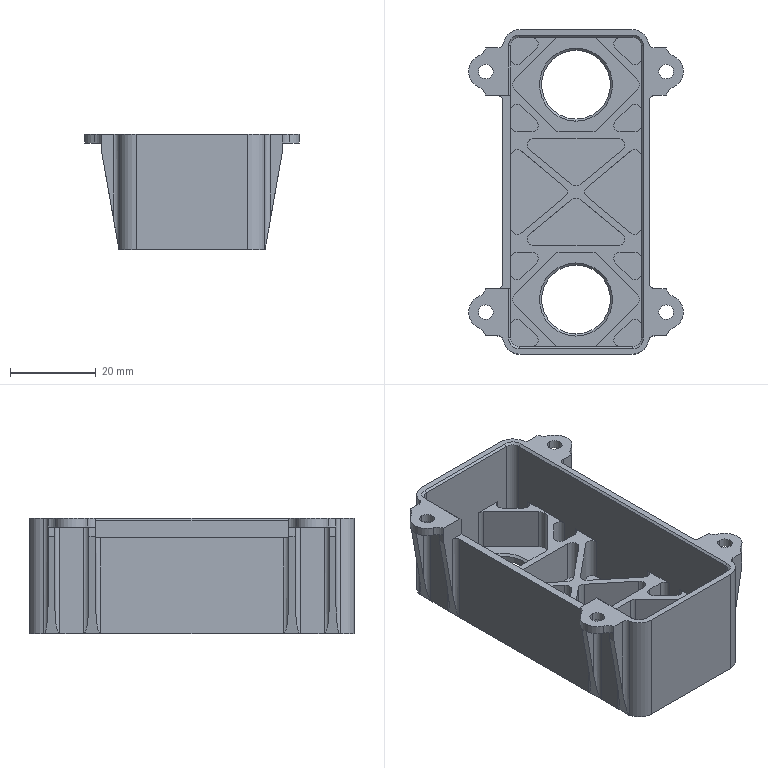NC program | NX | posted with a generic post | part box 50 x 75.58 x 26.8 mm
Lines 71 to 1246 of 35818:
(FLOOR_WALL , TOOL : D10)
N128 T15 M6
N130 G54
N132 G17 G0 G90 X23. Y1.305 S9500 M3
N134 G43 Z30. H15
N136 Z0.6
N138 G94 G1 Z-0.4 F1000.
N140 X22.357 Y0.766
N142 G3 X22. Y0. R1.
N144 G1 Y-17.499 F2000.
N146 G3 X21. Y-17.4 R5.1
N148 G1 X10.2
N150 Y17.4
N152 X21.
N154 G3 X22. Y17.499 R5.1
N156 G1 Y0.
N158 X17.
N160 Y-12.4
N162 X15.2
N164 Y12.4
N166 X17.
N168 Y0.
N170 G3 X17.357 Y-0.766 R1.
N172 G1 Z0.6
N174 G0 X23. Y1.305 Z0.2
N176 G1 Z-0.8 F1000.
N178 X22.357 Y0.766
N180 G3 X22. Y0. R1.
N182 G1 Y-17.499 F2000.
N184 G3 X21. Y-17.4 R5.1
N186 G1 X10.2
N188 Y17.4
N190 X21.
N192 G3 X22. Y17.499 R5.1
N194 G1 Y0.
N196 X17.
N198 Y-12.4
N200 X15.2
N202 Y12.4
N204 X17.
N206 Y0.
N208 G3 X17.357 Y-0.766 R1.
N210 G1 Z0.2
N212 G0 X23. Y1.305 Z-0.2
N214 G1 Z-1.2 F1000.
N216 X22.357 Y0.766
N218 G3 X22. Y0. R1.
N220 G1 Y-17.499 F2000.
N222 G3 X21. Y-17.4 R5.1
N224 G1 X10.2
N226 Y17.4
N228 X21.
N230 G3 X22. Y17.499 R5.1
N232 G1 Y0.
N234 X17.
N236 Y-12.4
N238 X15.2
N240 Y12.4
N242 X17.
N244 Y0.
N246 G3 X17.357 Y-0.766 R1.
N248 G1 Z-0.2
N250 G0 X23. Y1.305 Z-0.6
N252 G1 Z-1.6 F1000.
N254 X22.357 Y0.766
N256 G3 X22. Y0. R1.
N258 G1 Y-17.499 F2000.
N260 G3 X21. Y-17.4 R5.1
N262 G1 X10.2
N264 Y17.4
N266 X21.
N268 G3 X22. Y17.499 R5.1
N270 G1 Y0.
N272 X17.
N274 Y-12.4
N276 X15.2
N278 Y12.4
N280 X17.
N282 Y0.
N284 G3 X17.357 Y-0.766 R1.
N286 G1 Z-0.6
N288 G0 X23. Y1.305 Z-1.
N290 G1 Z-2. F1000.
N292 X22.357 Y0.766
N294 G3 X22. Y0. R1.
N296 G1 Y-17.499 F2000.
N298 G3 X21. Y-17.4 R5.1
N300 G1 X10.2
N302 Y17.4
N304 X21.
N306 G3 X22. Y17.499 R5.1
N308 G1 Y0.
N310 X17.
N312 Y-12.4
N314 X15.2
N316 Y12.4
N318 X17.
N320 Y0.
N322 G3 X17.357 Y-0.766 R1.
N324 G1 Z-1.
N326 G0 X23. Y1.305 Z-1.4
N328 G1 Z-2.4 F1000.
N330 X22.357 Y0.766
N332 G3 X22. Y0. R1.
N334 G1 Y-17.499 F2000.
N336 G3 X21. Y-17.4 R5.1
N338 G1 X10.2
N340 Y17.4
N342 X21.
N344 G3 X22. Y17.499 R5.1
N346 G1 Y0.
N348 X17.
N350 Y-12.4
N352 X15.2
N354 Y12.4
N356 X17.
N358 Y0.
N360 G3 X17.357 Y-0.766 R1.
N362 G1 Z-1.4
N364 G0 X23. Y1.305 Z-1.8
N366 G1 Z-2.8 F1000.
N368 X22.357 Y0.766
N370 G3 X22. Y0. R1.
N372 G1 Y-17.499 F2000.
N374 G3 X21. Y-17.4 R5.1
N376 G1 X10.2
N378 Y17.4
N380 X21.
N382 G3 X22. Y17.499 R5.1
N384 G1 Y0.
N386 X17.
N388 Y-12.4
N390 X15.2
N392 Y12.4
N394 X17.
N396 Y0.
N398 G3 X17.357 Y-0.766 R1.
N400 G1 Z-1.8
N402 G0 X23. Y1.305 Z-2.2
N404 G1 Z-3.2 F1000.
N406 X22.357 Y0.766
N408 G3 X22. Y0. R1.
N410 G1 Y-17.499 F2000.
N412 G3 X21. Y-17.4 R5.1
N414 G1 X10.2
N416 Y17.4
N418 X21.
N420 G3 X22. Y17.499 R5.1
N422 G1 Y0.
N424 X17.
N426 Y-12.4
N428 X15.2
N430 Y12.4
N432 X17.
N434 Y0.
N436 G3 X17.357 Y-0.766 R1.
N438 G1 Z-2.2
N440 G0 X23. Y1.305 Z-2.6
N442 G1 Z-3.6 F1000.
N444 X22.357 Y0.766
N446 G3 X22. Y0. R1.
N448 G1 Y-17.499 F2000.
N450 G3 X21. Y-17.4 R5.1
N452 G1 X10.2
N454 Y17.4
N456 X21.
N458 G3 X22. Y17.499 R5.1
N460 G1 Y0.
N462 X17.
N464 Y-12.4
N466 X15.2
N468 Y12.4
N470 X17.
N472 Y0.
N474 G3 X17.357 Y-0.766 R1.
N476 G1 Z-2.6
N478 G0 X23. Y1.305 Z-3.
N480 G1 Z-4. F1000.
N482 X22.357 Y0.766
N484 G3 X22. Y0. R1.
N486 G1 Y-17.499 F2000.
N488 G3 X21. Y-17.4 R5.1
N490 G1 X10.2
N492 Y17.4
N494 X21.
N496 G3 X22. Y17.499 R5.1
N498 G1 Y0.
N500 X17.
N502 Y-12.4
N504 X15.2
N506 Y12.4
N508 X17.
N510 Y0.
N512 G3 X17.357 Y-0.766 R1.
N514 G1 Z-3.
N516 G0 X23. Y1.305 Z-3.4
N518 G1 Z-4.4 F1000.
N520 X22.357 Y0.766
N522 G3 X22. Y0. R1.
N524 G1 Y-17.499 F2000.
N526 G3 X21. Y-17.4 R5.1
N528 G1 X10.2
N530 Y17.4
N532 X21.
N534 G3 X22. Y17.499 R5.1
N536 G1 Y0.
N538 X17.
N540 Y-12.4
N542 X15.2
N544 Y12.4
N546 X17.
N548 Y0.
N550 G3 X17.357 Y-0.766 R1.
N552 G1 Z-3.4
N554 G0 Z30.
(CAVITY_MILL_COPY_1 , TOOL : D10)
N556 X3.7 Y3.037
N558 Z1.5
N560 G1 Y9.845 Z1.143 F1000.
N562 X2.95 Y10.526 Z1.09
N564 X2.537 Y10.964 Z1.059
N566 X1.9 Y11.752 Z1.005
N568 Y-11.752 Z-0.226
N570 X2.537 Y-10.964 Z-0.279
N572 X2.95 Y-10.526 Z-0.311
N574 X3.7 Y-9.845 Z-0.364
N576 Y0. Z-0.88
N578 Y9.845 F2500.
N580 G2 X1.9 Y11.752 R17.1
N582 G1 Y-11.752
N584 G2 X3.7 Y-9.845 R17.1
N586 G1 Y0.
N588 X9.7
N590 Y12.858
N592 G2 X4.1 Y22.5 R11.1
N594 G1 Y24.89
N596 X-4.1
N598 Y-24.89
N600 X4.1
N602 Y-22.5
N604 G2 X9.7 Y-12.858 R11.1
N606 G1 Y0.
N608 X15.7
N610 Y17.4
N612 X15.2
N614 G2 X10.1 Y22.5 R5.1
N616 G1 Y30.89
N618 X-10.1
N620 Y-30.89
N622 X10.1
N624 Y-22.5
N626 G2 X15.2 Y-17.4 R5.1
N628 G1 X15.7
N630 Y0.
N632 G2 X16.2 Y0.866 R1.
N634 G1 Z0.12
N636 G0 Z30.
N638 X3.7 Y3.037
N640 Z0.62
N642 G1 Y9.845 Z0.263 F1000.
N644 X2.95 Y10.526 Z0.21
N646 X2.537 Y10.964 Z0.179
N648 X1.9 Y11.752 Z0.125
N650 Y-11.752 Z-1.106
N652 X2.537 Y-10.964 Z-1.159
N654 X2.95 Y-10.526 Z-1.191
N656 X3.7 Y-9.845 Z-1.244
N658 Y0. Z-1.76
N660 Y9.845 F2500.
N662 G2 X1.9 Y11.752 R17.1
N664 G1 Y-11.752
N666 G2 X3.7 Y-9.845 R17.1
N668 G1 Y0.
N670 X9.7
N672 Y12.858
N674 G2 X4.1 Y22.5 R11.1
N676 G1 Y24.89
N678 X-4.1
N680 Y-24.89
N682 X4.1
N684 Y-22.5
N686 G2 X9.7 Y-12.858 R11.1
N688 G1 Y0.
N690 X15.7
N692 Y17.4
N694 X15.2
N696 G2 X10.1 Y22.5 R5.1
N698 G1 Y30.89
N700 X-10.1
N702 Y-30.89
N704 X10.1
N706 Y-22.5
N708 G2 X15.2 Y-17.4 R5.1
N710 G1 X15.7
N712 Y0.
N714 G2 X16.2 Y0.866 R1.
N716 G1 Z-0.76
N718 G0 X3.7 Y3.037 Z-0.26
N720 G1 Y9.845 Z-0.617 F1000.
N722 X2.95 Y10.526 Z-0.67
N724 X2.537 Y10.964 Z-0.701
N726 X1.9 Y11.752 Z-0.755
N728 Y-11.752 Z-1.986
N730 X2.537 Y-10.964 Z-2.039
N732 X2.95 Y-10.526 Z-2.071
N734 X3.7 Y-9.845 Z-2.124
N736 Y0. Z-2.64
N738 Y9.845 F2500.
N740 G2 X1.9 Y11.752 R17.1
N742 G1 Y-11.752
N744 G2 X3.7 Y-9.845 R17.1
N746 G1 Y0.
N748 X9.7
N750 Y12.858
N752 G2 X4.1 Y22.5 R11.1
N754 G1 Y24.89
N756 X-4.1
N758 Y-24.89
N760 X4.1
N762 Y-22.5
N764 G2 X9.7 Y-12.858 R11.1
N766 G1 Y0.
N768 X15.7
N770 Y17.4
N772 X15.2
N774 G2 X10.1 Y22.5 R5.1
N776 G1 Y30.89
N778 X-10.1
N780 Y-30.89
N782 X10.1
N784 Y-22.5
N786 G2 X15.2 Y-17.4 R5.1
N788 G1 X15.7
N790 Y0.
N792 G2 X16.2 Y0.866 R1.
N794 G1 Z-1.64
N796 G0 X3.7 Y3.037 Z-1.14
N798 G1 Y9.845 Z-1.497 F1000.
N800 X2.95 Y10.526 Z-1.55
N802 X2.537 Y10.964 Z-1.581
N804 X1.9 Y11.752 Z-1.635
N806 Y-11.752 Z-2.866
N808 X2.537 Y-10.964 Z-2.919
N810 X2.95 Y-10.526 Z-2.951
N812 X3.7 Y-9.845 Z-3.004
N814 Y0. Z-3.52
N816 Y9.845 F2500.
N818 G2 X1.9 Y11.752 R17.1
N820 G1 Y-11.752
N822 G2 X3.7 Y-9.845 R17.1
N824 G1 Y0.
N826 X9.7
N828 Y12.858
N830 G2 X4.1 Y22.5 R11.1
N832 G1 Y24.89
N834 X-4.1
N836 Y-24.89
N838 X4.1
N840 Y-22.5
N842 G2 X9.7 Y-12.858 R11.1
N844 G1 Y0.
N846 X15.7
N848 Y17.4
N850 X15.2
N852 G2 X10.1 Y22.5 R5.1
N854 G1 Y30.89
N856 X-10.1
N858 Y-30.89
N860 X10.1
N862 Y-22.5
N864 G2 X15.2 Y-17.4 R5.1
N866 G1 X15.7
N868 Y0.
N870 G2 X16.2 Y0.866 R1.
N872 G1 Z-2.52
N874 G0 X3.7 Y3.037 Z-2.02
N876 G1 Y9.845 Z-2.377 F1000.
N878 X2.95 Y10.526 Z-2.43
N880 X2.537 Y10.964 Z-2.461
N882 X1.9 Y11.752 Z-2.515
N884 Y-11.752 Z-3.746
N886 X2.537 Y-10.964 Z-3.799
N888 X2.95 Y-10.526 Z-3.831
N890 X3.7 Y-9.845 Z-3.884
N892 Y0. Z-4.4
N894 Y9.845 F2500.
N896 G2 X1.9 Y11.752 R17.1
N898 G1 Y-11.752
N900 G2 X3.7 Y-9.845 R17.1
N902 G1 Y0.
N904 X9.7
N906 Y12.858
N908 G2 X4.1 Y22.5 R11.1
N910 G1 Y24.89
N912 X-4.1
N914 Y-24.89
N916 X4.1
N918 Y-22.5
N920 G2 X9.7 Y-12.858 R11.1
N922 G1 Y0.
N924 X15.7
N926 Y17.4
N928 X15.2
N930 G2 X10.1 Y22.5 R5.1
N932 G1 Y30.89
N934 X-10.1
N936 Y-30.89
N938 X10.1
N940 Y-22.5
N942 G2 X15.2 Y-17.4 R5.1
N944 G1 X15.7
N946 Y0.
N948 G2 X16.2 Y0.866 R1.
N950 G1 Z-3.4
N952 G0 X4.1 Y11.491 Z-2.9
N954 G1 Y24.89 Z-3.602 F1000.
N956 X-4.1 Z-4.032
N958 Y0. Z-5.336
N960 Y-24.89 F2500.
N962 X4.1
N964 Y24.89
N966 X-4.1
N968 Y0.
N970 X-10.1
N972 Y-30.89
N974 X10.1
N976 Y30.89
N978 X-10.1
N980 Y0.
N982 G3 X-9.6 Y-0.866 R1.
N984 G1 Z-4.336
N986 G0 X4.1 Y11.491 Z-3.836
N988 G1 Y24.89 Z-4.539 F1000.
N990 X-4.1 Z-4.968
N992 Y0. Z-6.273
N994 Y-24.89 F2500.
N996 X4.1
N998 Y24.89
N1000 X-4.1
N1002 Y0.
N1004 X-10.1
N1006 Y-30.89
N1008 X10.1
N1010 Y30.89
N1012 X-10.1
N1014 Y0.
N1016 G3 X-9.6 Y-0.866 R1.
N1018 G1 Z-5.273
N1020 G0 X4.1 Y11.497 Z-4.773
N1022 G1 Y24.89 Z-5.475 F1000.
N1024 X-4.1 Z-5.904
N1026 Y7.945 Z-6.792
N1028 X-4.04 Y7.337 Z-6.824
N1030 X-4.1 Y6.739 Z-6.856
N1032 Y0. Z-7.209
N1034 Y-6.739 F2500.
N1036 G2 X-4.1 Y-7.945 R6.
N1038 G1 Y-24.89
N1040 X4.1
N1042 Y24.89
N1044 X-4.1
N1046 Y7.945
N1048 G2 X-4.1 Y6.739 R6.
N1050 G1 Y0.
N1052 X-10.1
N1054 Y-7.242
N1056 X-10.07 Y-7.342
N1058 X-10.1 Y-7.39
N1060 Y-30.89
N1062 X10.1
N1064 Y30.89
N1066 X-10.1
N1068 Y7.39
N1070 X-10.07 Y7.342
N1072 X-10.1 Y7.242
N1074 Y0.
N1076 G3 X-9.6 Y-0.866 R1.
N1078 G1 Z-6.209
N1080 G0 X4.1 Y11.498 Z-5.709
N1082 G1 Y24.89 Z-6.411 F1000.
N1084 X-4.1 Z-6.841
N1086 Y7.987 Z-7.727
N1088 X-4.035 Y7.389 Z-7.758
N1090 Y7.295 Z-7.763
N1092 X-4.1 Y6.698 Z-7.794
N1094 Y0. Z-8.145
N1096 Y-6.698 F2500.
N1098 G2 X-4.1 Y-7.987 R6.
N1100 G1 Y-24.89
N1102 X4.1
N1104 Y24.89
N1106 X-4.1
N1108 Y7.987
N1110 G2 X-4.1 Y6.698 R6.
N1112 G1 Y0.
N1114 X-10.1
N1116 Y-7.242
N1118 X-10.065 Y-7.342
N1120 X-10.1 Y-7.39
N1122 Y-30.89
N1124 X10.1
N1126 Y30.89
N1128 X-10.1
N1130 Y7.39
N1132 X-10.065 Y7.342
N1134 X-10.1 Y7.242
N1136 Y0.
N1138 G3 X-9.6 Y-0.866 R1.
N1140 G1 Z-7.145
N1142 G0 X-4.1 Y-11.491 Z-6.645
N1144 G1 Y-24.89 Z-7.348 F1000.
N1146 X4.1 Z-7.777
N1148 Y0. Z-9.082
N1150 Y24.89 F2500.
N1152 X-4.1
N1154 Y8.025
N1156 G2 X-4.1 Y6.659 R6.
N1158 G1 Y-6.659
N1160 G2 X-4.1 Y-8.025 R6.
N1162 G1 Y-24.89
N1164 X4.1
N1166 Y0.
N1168 X10.1
N1170 Y30.89
N1172 X-10.1
N1174 Y7.39
N1176 X-10.061 Y7.342
N1178 X-10.1 Y7.242
N1180 Y-7.242
N1182 X-10.061 Y-7.342
N1184 X-10.1 Y-7.39
N1186 Y-30.89
N1188 X10.1
N1190 Y0.
N1192 G3 X9.6 Y0.866 R1.
N1194 G1 Z-8.082
N1196 G0 X-4.1 Y-11.491 Z-7.582
N1198 G1 Y-24.89 Z-8.284 F1000.
N1200 X4.1 Z-8.714
N1202 Y0. Z-10.018
N1204 Y24.89 F2500.
N1206 X-4.1
N1208 Y8.062
N1210 G2 X-4.1 Y6.622 R6.
N1212 G1 Y-6.622
N1214 G2 X-4.1 Y-8.062 R6.
N1216 G1 Y-24.89
N1218 X4.1
N1220 Y0.
N1222 X10.1
N1224 Y30.89
N1226 X-10.1
N1228 Y7.39
N1230 X-10.057 Y7.342
N1232 X-10.1 Y7.242
N1234 Y-7.242
N1236 X-10.057 Y-7.342
N1238 X-10.1 Y-7.39
N1240 Y-30.89
N1242 X10.1
N1244 Y0.
N1246 G3 X9.6 Y0.866 R1.
N1248 G1 Z-9.018
N1250 G0 X-4.1 Y-11.491 Z-8.518
N1252 G1 Y-24.89 Z-9.22 F1000.
N1254 X4.1 Z-9.65
N1256 Y0. Z-10.955
N1258 Y24.89 F2500.
N1260 X-4.1
N1262 Y8.097
N1264 G2 X-4.1 Y6.587 R6.
N1266 G1 Y-6.587
N1268 G2 X-4.1 Y-8.097 R6.
N1270 G1 Y-24.89
N1272 X4.1
N1274 Y0.
N1276 X10.1
N1278 Y30.89
N1280 X-10.1
N1282 Y7.39
N1284 X-10.052 Y7.342
N1286 X-10.1 Y7.242
N1288 Y-7.242
N1290 X-10.052 Y-7.342
N1292 X-10.1 Y-7.39
N1294 Y-30.89
N1296 X10.1
N1298 Y0.
N1300 G3 X9.6 Y0.866 R1.
N1302 G1 Z-9.955
N1304 G0 X-4.1 Y-11.491 Z-9.455
N1306 G1 Y-24.89 Z-10.157 F1000.
N1308 X4.1 Z-10.586
N1310 Y0. Z-11.891
N1312 Y24.89 F2500.
N1314 X-4.1
N1316 Y8.13
N1318 G2 X-4.1 Y6.554 R6.
N1320 G1 Y-6.554
N1322 G2 X-4.1 Y-8.13 R6.
N1324 G1 Y-24.89
N1326 X4.1
N1328 Y0.
N1330 X10.1
N1332 Y30.89
N1334 X-10.1
N1336 Y7.39
N1338 X-10.048 Y7.342
N1340 X-10.1 Y7.242
N1342 Y-7.242
N1344 X-10.048 Y-7.342
N1346 X-10.1 Y-7.39
N1348 Y-30.89
N1350 X10.1
N1352 Y0.
N1354 G3 X9.6 Y0.866 R1.
N1356 G1 Z-10.891
N1358 G0 X4.1 Y11.5 Z-10.391
N1360 G1 Y24.89 Z-11.093 F1000.
N1362 X-4.1 Z-11.522
N1364 Y8.174 Z-12.398
N1366 X-4.039 Y7.747 Z-12.421
N1368 Y6.885 Z-12.466
N1370 X-4.1 Y6.459 Z-12.489
N1372 Y0. Z-12.827
N1374 Y-6.459 F2500.
N1376 G2 X-4.1 Y-8.174 R6.076
N1378 G1 Y-24.89
N1380 X4.1
N1382 Y24.89
N1384 X-4.1
N1386 Y8.174
N1388 G2 X-4.1 Y6.459 R6.076
N1390 G1 Y0.
N1392 X-10.1
N1394 Y-7.242
N1396 G2 X-10.1 Y-7.39 R0.076
N1398 G1 Y-30.89
N1400 X10.1
N1402 Y30.89
N1404 X-10.1
N1406 Y7.39
N1408 G2 X-10.1 Y7.242 R0.076
N1410 G1 Y0.
N1412 G3 X-9.6 Y-0.866 R1.
N1414 G1 Z-11.827
N1416 G0 X4.1 Y11.501 Z-11.327
N1418 G1 Y24.89 Z-12.029 F1000.
N1420 X-4.1 Z-12.459
N1422 Y8.204 Z-13.333
N1424 X-4.035 Y7.763 Z-13.357
N1426 Y6.87 Z-13.403
N1428 X-4.1 Y6.428 Z-13.427
N1430 Y0. Z-13.764
N1432 Y-6.428 F2500.
N1434 G2 X-4.1 Y-8.204 R6.075
N1436 G1 Y-24.89
N1438 X4.1
N1440 Y24.89
N1442 X-4.1
N1444 Y8.204
N1446 G2 X-4.1 Y6.428 R6.075
N1448 G1 Y0.
N1450 X-10.1
N1452 Y-7.242
N1454 G2 X-10.1 Y-7.39 R0.075
N1456 G1 Y-30.89
N1458 X10.1
N1460 Y30.89
N1462 X-10.1
N1464 Y7.39
N1466 G2 X-10.1 Y7.242 R0.075
N1468 G1 Y0.
N1470 G3 X-9.6 Y-0.866 R1.
N1472 G1 Z-12.764
N1474 G0 X4.1 Y11.502 Z-12.264
N1476 G1 Y24.89 Z-12.965 F1000.
N1478 X-4.1 Z-13.395
N1480 Y8.233 Z-14.268
N1482 X-4.03 Y7.777 Z-14.292
N1484 Y6.855 Z-14.34
N1486 X-4.1 Y6.4 Z-14.365
N1488 Y0. Z-14.7
N1490 Y-6.4 F2500.
N1492 G2 X-4.1 Y-8.233 R6.074
N1494 G1 Y-24.89
N1496 X4.1
N1498 Y24.89
N1500 X-4.1
N1502 Y8.233
N1504 G2 X-4.1 Y6.4 R6.074
N1506 G1 Y0.
N1508 X-10.1
N1510 Y-7.242
N1512 G2 X-10.1 Y-7.39 R0.074
N1514 G1 Y-30.89
N1516 X10.1
N1518 Y30.89
N1520 X-10.1
N1522 Y7.39
N1524 G2 X-10.1 Y7.242 R0.074
N1526 G1 Y0.
N1528 G3 X-9.6 Y-0.866 R1.
N1530 G1 Z-13.7
N1532 G0 X-0.363 Y-26.39 Z-13.2
N1534 G1 X0.576 Z-13.249 F1000.
N1536 X1.966 Y-25. Z-13.352
N1538 X0.566 Y-23.6 Z-13.456
N1540 X-0.566 Z-13.515
N1542 X-1.966 Y-25. Z-13.619
N1544 X-0.576 Y-26.39 Z-13.722
N1546 X0.576 Z-13.782
N1548 X1.966 Y-25. Z-13.885
N1550 X0.566 Y-23.6 Z-13.989
N1552 X-0.566 Z-14.048
N1554 X-1.966 Y-25. Z-14.152
N1556 X-0.576 Y-26.39 Z-14.255
N1558 X0.576 Z-14.316
N1560 X1.966 Y-25. Z-14.419
N1562 X0.566 Y-23.6 Z-14.522
N1564 X-0.566 Z-14.582
N1566 X-1.966 Y-25. Z-14.685
N1568 X-0.576 Y-26.39 Z-14.788
N1570 X0.576 Z-14.849
N1572 X1.966 Y-25. Z-14.952
N1574 X0.566 Y-23.6 Z-15.056
N1576 X-0.566 Z-15.115
N1578 X-1.966 Y-25. Z-15.219
N1580 X-0.576 Y-26.39 Z-15.322
N1582 X0.576 Z-15.382
N1584 X1.966 Y-25. Z-15.485
N1586 X0.566 Y-23.6 Z-15.589
N1588 X-0.566 Z-15.648
N1590 X-1.266 Y-24.3 Z-15.7
N1592 X-1.966 Y-25. F2500.
N1594 X-0.576 Y-26.39
N1596 X0.576
N1598 X1.966 Y-25.
N1600 X0.566 Y-23.6
N1602 X-0.566
N1604 X-1.266 Y-24.3
N1606 X-4.448 Y-21.118
N1608 X-8.33 Y-25.
N1610 X-2.44 Y-30.89
N1612 X2.44
N1614 X8.33 Y-25.
N1616 X2.43 Y-19.1
N1618 X-2.43
N1620 X-4.448 Y-21.118
N1622 G3 X-4.707 Y-22.084 R1.
N1624 G1 Z-14.7
N1626 G0 X-0.363 Y-26.39 Z-14.2
N1628 G1 X0.576 Z-14.249 F1000.
N1630 X1.966 Y-25. Z-14.352
N1632 X0.566 Y-23.6 Z-14.456
N1634 X-0.566 Z-14.515
N1636 X-1.966 Y-25. Z-14.619
N1638 X-0.576 Y-26.39 Z-14.722
N1640 X0.576 Z-14.782
N1642 X1.966 Y-25. Z-14.885
N1644 X0.566 Y-23.6 Z-14.989
N1646 X-0.566 Z-15.048
N1648 X-1.966 Y-25. Z-15.152
N1650 X-0.576 Y-26.39 Z-15.255
N1652 X0.576 Z-15.316
N1654 X1.966 Y-25. Z-15.419
N1656 X0.566 Y-23.6 Z-15.522
N1658 X-0.566 Z-15.582
N1660 X-1.966 Y-25. Z-15.685
N1662 X-0.576 Y-26.39 Z-15.788
N1664 X0.576 Z-15.849
N1666 X1.966 Y-25. Z-15.952
N1668 X0.566 Y-23.6 Z-16.056
N1670 X-0.566 Z-16.115
N1672 X-1.966 Y-25. Z-16.219
N1674 X-0.576 Y-26.39 Z-16.322
N1676 X0.576 Z-16.382
N1678 X1.966 Y-25. Z-16.485
N1680 X0.566 Y-23.6 Z-16.589
N1682 X-0.566 Z-16.648
N1684 X-1.266 Y-24.3 Z-16.7
N1686 X-1.966 Y-25. F2500.
N1688 X-0.576 Y-26.39
N1690 X0.576
N1692 X1.966 Y-25.
N1694 X0.566 Y-23.6
N1696 X-0.566
N1698 X-1.266 Y-24.3
N1700 X-4.448 Y-21.118
N1702 X-8.33 Y-25.
N1704 X-2.44 Y-30.89
N1706 X2.44
N1708 X8.33 Y-25.
N1710 X2.43 Y-19.1
N1712 X-2.43
N1714 X-4.448 Y-21.118
N1716 G3 X-4.707 Y-22.084 R1.
N1718 G1 Z-15.7
N1720 G0 X-1.306 Y-24.341 Z-15.2
N1722 G1 X-1.966 Y-25. Z-15.249 F1000.
N1724 X-0.576 Y-26.39 Z-15.352
N1726 X0.576 Z-15.412
N1728 X1.966 Y-25. Z-15.515
N1730 X0.566 Y-23.6 Z-15.619
N1732 X-0.566 Z-15.678
N1734 X-1.966 Y-25. Z-15.782
N1736 X-0.576 Y-26.39 Z-15.885
N1738 X0.576 Z-15.945
N1740 X1.966 Y-25. Z-16.048
N1742 X0.566 Y-23.6 Z-16.152
N1744 X-0.566 Z-16.212
N1746 X-1.966 Y-25. Z-16.315
N1748 X-0.576 Y-26.39 Z-16.418
N1750 X0.576 Z-16.479
N1752 X1.966 Y-25. Z-16.582
N1754 X0.566 Y-23.6 Z-16.685
N1756 X-0.566 Z-16.745
N1758 X-1.966 Y-25. Z-16.849
N1760 X-0.576 Y-26.39 Z-16.952
N1762 X0.576 Z-17.012
N1764 X1.966 Y-25. Z-17.115
N1766 X0.566 Y-23.6 Z-17.219
N1768 X-0.566 Z-17.278
N1770 X-1.966 Y-25. Z-17.382
N1772 X-0.576 Y-26.39 Z-17.485
N1774 X0.576 Z-17.545
N1776 X1.966 Y-25. Z-17.648
N1778 X1.266 Y-24.3 Z-17.7
N1780 X0.566 Y-23.6 F2500.
N1782 X-0.566
N1784 X-1.966 Y-25.
N1786 X-0.576 Y-26.39
N1788 X0.576
N1790 X1.966 Y-25.
N1792 X1.266 Y-24.3
N1794 X4.448 Y-21.118
N1796 X2.429 Y-19.1
N1798 X-2.43
N1800 X-8.33 Y-25.
N1802 X-2.44 Y-30.89
N1804 X2.44
N1806 X8.33 Y-25.
N1808 X4.448 Y-21.118
N1810 G3 X3.482 Y-20.859 R1.
N1812 G1 Z-16.7
N1814 G0 X-1.306 Y-24.341 Z-16.2
N1816 G1 X-1.966 Y-25. Z-16.249 F1000.
N1818 X-0.576 Y-26.39 Z-16.352
N1820 X0.576 Z-16.412
N1822 X1.966 Y-25. Z-16.515
N1824 X0.566 Y-23.6 Z-16.619
N1826 X-0.566 Z-16.678
N1828 X-1.966 Y-25. Z-16.782
N1830 X-0.576 Y-26.39 Z-16.885
N1832 X0.576 Z-16.945
N1834 X1.966 Y-25. Z-17.048
N1836 X0.566 Y-23.6 Z-17.152
N1838 X-0.566 Z-17.212
N1840 X-1.966 Y-25. Z-17.315
N1842 X-0.576 Y-26.39 Z-17.418
N1844 X0.576 Z-17.479
N1846 X1.966 Y-25. Z-17.582
N1848 X0.566 Y-23.6 Z-17.685
N1850 X-0.566 Z-17.745
N1852 X-1.966 Y-25. Z-17.849
N1854 X-0.576 Y-26.39 Z-17.952
N1856 X0.576 Z-18.012
N1858 X1.966 Y-25. Z-18.115
N1860 X0.566 Y-23.6 Z-18.219
N1862 X-0.566 Z-18.278
N1864 X-1.966 Y-25. Z-18.382
N1866 X-0.576 Y-26.39 Z-18.485
N1868 X0.576 Z-18.545
N1870 X1.966 Y-25. Z-18.648
N1872 X1.266 Y-24.3 Z-18.7
N1874 X0.566 Y-23.6 F2500.
N1876 X-0.566
N1878 X-1.966 Y-25.
N1880 X-0.576 Y-26.39
N1882 X0.576
N1884 X1.966 Y-25.
N1886 X1.266 Y-24.3
N1888 X4.448 Y-21.118
N1890 X2.429 Y-19.1
N1892 X-2.43
N1894 X-8.33 Y-25.
N1896 X-2.44 Y-30.89
N1898 X2.44
N1900 X8.33 Y-25.
N1902 X4.448 Y-21.118
N1904 G3 X3.482 Y-20.859 R1.
N1906 G1 Z-17.7
N1908 G0 X-0.363 Y-26.39 Z-17.2
N1910 G1 X0.576 Z-17.249 F1000.
N1912 X1.966 Y-25. Z-17.352
N1914 X0.566 Y-23.6 Z-17.456
N1916 X-0.566 Z-17.515
N1918 X-1.966 Y-25. Z-17.619
N1920 X-0.576 Y-26.39 Z-17.722
N1922 X0.576 Z-17.782
N1924 X1.966 Y-25. Z-17.885
N1926 X0.566 Y-23.6 Z-17.989
N1928 X-0.566 Z-18.048
N1930 X-1.966 Y-25. Z-18.152
N1932 X-0.576 Y-26.39 Z-18.255
N1934 X0.576 Z-18.316
N1936 X1.966 Y-25. Z-18.419
N1938 X0.566 Y-23.6 Z-18.522
N1940 X-0.566 Z-18.582
N1942 X-1.966 Y-25. Z-18.685
N1944 X-0.576 Y-26.39 Z-18.788
N1946 X0.576 Z-18.849
N1948 X1.966 Y-25. Z-18.952
N1950 X0.566 Y-23.6 Z-19.056
N1952 X-0.566 Z-19.115
N1954 X-1.966 Y-25. Z-19.219
N1956 X-0.576 Y-26.39 Z-19.322
N1958 X0.576 Z-19.382
N1960 X1.966 Y-25. Z-19.485
N1962 X0.566 Y-23.6 Z-19.589
N1964 X-0.566 Z-19.648
N1966 X-1.266 Y-24.3 Z-19.7
N1968 X-1.966 Y-25. F2500.
N1970 X-0.576 Y-26.39
N1972 X0.576
N1974 X1.966 Y-25.
N1976 X0.566 Y-23.6
N1978 X-0.566
N1980 X-1.266 Y-24.3
N1982 X-4.448 Y-21.118
N1984 X-8.33 Y-25.
N1986 X-2.44 Y-30.89
N1988 X2.44
N1990 X8.33 Y-25.
N1992 X2.429 Y-19.1
N1994 X-2.43
N1996 X-4.448 Y-21.118
N1998 G3 X-4.707 Y-22.084 R1.
N2000 G1 Z-18.7
N2002 G0 X-0.363 Y-26.39 Z-18.2
N2004 G1 X0.576 Z-18.249 F1000.
N2006 X1.966 Y-25. Z-18.352
N2008 X0.566 Y-23.6 Z-18.456
N2010 X-0.566 Z-18.515
N2012 X-1.966 Y-25. Z-18.619
N2014 X-0.576 Y-26.39 Z-18.722
N2016 X0.576 Z-18.782
N2018 X1.966 Y-25. Z-18.885
N2020 X0.566 Y-23.6 Z-18.989
N2022 X-0.566 Z-19.048
N2024 X-1.966 Y-25. Z-19.152
N2026 X-0.576 Y-26.39 Z-19.255
N2028 X0.576 Z-19.316
N2030 X1.966 Y-25. Z-19.419
N2032 X0.566 Y-23.6 Z-19.522
N2034 X-0.566 Z-19.582
N2036 X-1.966 Y-25. Z-19.685
N2038 X-0.576 Y-26.39 Z-19.788
N2040 X0.576 Z-19.849
N2042 X1.966 Y-25. Z-19.952
N2044 X0.566 Y-23.6 Z-20.056
N2046 X-0.566 Z-20.115
N2048 X-1.966 Y-25. Z-20.219
N2050 X-0.576 Y-26.39 Z-20.322
N2052 X0.576 Z-20.382
N2054 X1.966 Y-25. Z-20.485
N2056 X0.566 Y-23.6 Z-20.589
N2058 X-0.566 Z-20.648
N2060 X-1.266 Y-24.3 Z-20.7
N2062 X-1.966 Y-25. F2500.
N2064 X-0.576 Y-26.39
N2066 X0.576
N2068 X1.966 Y-25.
N2070 X0.566 Y-23.6
N2072 X-0.566
N2074 X-1.266 Y-24.3
N2076 X-4.448 Y-21.118
N2078 X-8.33 Y-25.
N2080 X-2.44 Y-30.89
N2082 X2.44
N2084 X8.33 Y-25.
N2086 X2.429 Y-19.1
N2088 X-2.43
N2090 X-4.448 Y-21.118
N2092 G3 X-4.707 Y-22.084 R1.
N2094 G1 Z-19.7
N2096 G0 X-0.363 Y-26.39 Z-19.2
N2098 G1 X0.576 Z-19.249 F1000.
N2100 X1.966 Y-25. Z-19.352
N2102 X0.566 Y-23.6 Z-19.456
N2104 X-0.566 Z-19.515
N2106 X-1.966 Y-25. Z-19.619
N2108 X-0.576 Y-26.39 Z-19.722
N2110 X0.576 Z-19.782
N2112 X1.966 Y-25. Z-19.885
N2114 X0.566 Y-23.6 Z-19.989
N2116 X-0.566 Z-20.048
N2118 X-1.966 Y-25. Z-20.152
N2120 X-0.576 Y-26.39 Z-20.255
N2122 X0.576 Z-20.316
N2124 X1.966 Y-25. Z-20.419
N2126 X0.566 Y-23.6 Z-20.522
N2128 X-0.566 Z-20.582
N2130 X-1.966 Y-25. Z-20.685
N2132 X-0.576 Y-26.39 Z-20.788
N2134 X0.576 Z-20.849
N2136 X1.966 Y-25. Z-20.952
N2138 X0.566 Y-23.6 Z-21.056
N2140 X-0.566 Z-21.115
N2142 X-1.966 Y-25. Z-21.219
N2144 X-0.576 Y-26.39 Z-21.322
N2146 X0.576 Z-21.382
N2148 X1.966 Y-25. Z-21.485
N2150 X0.566 Y-23.6 Z-21.589
N2152 X-0.566 Z-21.648
N2154 X-1.266 Y-24.3 Z-21.7
N2156 X-1.966 Y-25. F2500.
N2158 X-0.576 Y-26.39
N2160 X0.576
N2162 X1.966 Y-25.
N2164 X0.566 Y-23.6
N2166 X-0.566
N2168 X-1.266 Y-24.3
N2170 X-4.448 Y-21.118
N2172 X-8.33 Y-25.
N2174 X-2.44 Y-30.89
N2176 X2.44
N2178 X8.33 Y-25.
N2180 X2.429 Y-19.1
N2182 X-2.43
N2184 X-4.448 Y-21.118
N2186 G3 X-4.707 Y-22.084 R1.
N2188 G1 Z-20.7
N2190 G0 X-1.306 Y-24.341 Z-20.2
N2192 G1 X-1.966 Y-25. Z-20.249 F1000.
N2194 X-0.576 Y-26.39 Z-20.352
N2196 X0.576 Z-20.412
N2198 X1.966 Y-25. Z-20.515
N2200 X0.566 Y-23.6 Z-20.619
N2202 X-0.566 Z-20.678
N2204 X-1.966 Y-25. Z-20.782
N2206 X-0.576 Y-26.39 Z-20.885
N2208 X0.576 Z-20.945
N2210 X1.966 Y-25. Z-21.048
N2212 X0.566 Y-23.6 Z-21.152
N2214 X-0.566 Z-21.212
N2216 X-1.966 Y-25. Z-21.315
N2218 X-0.576 Y-26.39 Z-21.418
N2220 X0.576 Z-21.479
N2222 X1.966 Y-25. Z-21.582
N2224 X0.566 Y-23.6 Z-21.685
N2226 X-0.566 Z-21.745
N2228 X-1.966 Y-25. Z-21.849
N2230 X-0.576 Y-26.39 Z-21.952
N2232 X0.576 Z-22.012
N2234 X1.966 Y-25. Z-22.115
N2236 X0.566 Y-23.6 Z-22.219
N2238 X-0.566 Z-22.278
N2240 X-1.966 Y-25. Z-22.382
N2242 X-0.576 Y-26.39 Z-22.485
N2244 X0.576 Z-22.545
N2246 X1.966 Y-25. Z-22.648
N2248 X1.266 Y-24.3 Z-22.7
N2250 X0.566 Y-23.6 F2500.
N2252 X-0.566
N2254 X-1.966 Y-25.
N2256 X-0.576 Y-26.39
N2258 X0.576
N2260 X1.966 Y-25.
N2262 X1.266 Y-24.3
N2264 X4.448 Y-21.118
N2266 X2.429 Y-19.1
N2268 X-2.43
N2270 X-8.33 Y-25.
N2272 X-2.44 Y-30.89
N2274 X2.44
N2276 X8.33 Y-25.
N2278 X4.448 Y-21.118
N2280 G3 X3.482 Y-20.859 R1.
N2282 G1 Z-21.7
N2284 G0 X-1.306 Y-24.341 Z-21.2
N2286 G1 X-1.966 Y-25. Z-21.249 F1000.
N2288 X-0.576 Y-26.39 Z-21.352
N2290 X0.576 Z-21.412
N2292 X1.966 Y-25. Z-21.515
N2294 X0.566 Y-23.6 Z-21.619
N2296 X-0.566 Z-21.678
N2298 X-1.966 Y-25. Z-21.782
N2300 X-0.576 Y-26.39 Z-21.885
N2302 X0.576 Z-21.945
N2304 X1.966 Y-25. Z-22.048
N2306 X0.566 Y-23.6 Z-22.152
N2308 X-0.566 Z-22.212
N2310 X-1.966 Y-25. Z-22.315
N2312 X-0.576 Y-26.39 Z-22.418
N2314 X0.576 Z-22.479
N2316 X1.966 Y-25. Z-22.582
N2318 X0.566 Y-23.6 Z-22.685
N2320 X-0.566 Z-22.745
N2322 X-1.966 Y-25. Z-22.849
N2324 X-0.576 Y-26.39 Z-22.952
N2326 X0.576 Z-23.012
N2328 X1.966 Y-25. Z-23.115
N2330 X0.566 Y-23.6 Z-23.219
N2332 X-0.566 Z-23.278
N2334 X-1.966 Y-25. Z-23.382
N2336 X-0.576 Y-26.39 Z-23.485
N2338 X0.576 Z-23.545
N2340 X1.966 Y-25. Z-23.648
N2342 X1.266 Y-24.3 Z-23.7
N2344 X0.566 Y-23.6 F2500.
N2346 X-0.566
N2348 X-1.966 Y-25.
N2350 X-0.576 Y-26.39
N2352 X0.576
N2354 X1.966 Y-25.
N2356 X1.266 Y-24.3
N2358 X4.448 Y-21.118
N2360 X2.429 Y-19.1
N2362 X-2.43
N2364 X-8.33 Y-25.
N2366 X-2.44 Y-30.89
N2368 X2.44
N2370 X8.33 Y-25.
N2372 X4.448 Y-21.118
N2374 G3 X3.482 Y-20.859 R1.
N2376 G1 Z-22.7
N2378 G0 X-1.306 Y-24.341 Z-22.2
N2380 G1 X-1.966 Y-25. Z-22.249 F1000.
N2382 X-0.576 Y-26.39 Z-22.352
N2384 X0.576 Z-22.412
N2386 X1.966 Y-25. Z-22.515
N2388 X0.566 Y-23.6 Z-22.619
N2390 X-0.566 Z-22.678
N2392 X-1.966 Y-25. Z-22.782
N2394 X-0.576 Y-26.39 Z-22.885
N2396 X0.576 Z-22.945
N2398 X1.966 Y-25. Z-23.048
N2400 X0.566 Y-23.6 Z-23.152
N2402 X-0.566 Z-23.212
N2404 X-1.966 Y-25. Z-23.315
N2406 X-0.576 Y-26.39 Z-23.418
N2408 X0.576 Z-23.479
N2410 X1.966 Y-25. Z-23.582
N2412 X0.566 Y-23.6 Z-23.685
N2414 X-0.566 Z-23.745
N2416 X-1.966 Y-25. Z-23.849
N2418 X-0.576 Y-26.39 Z-23.952
N2420 X0.576 Z-24.012
N2422 X1.966 Y-25. Z-24.115
N2424 X0.566 Y-23.6 Z-24.219
N2426 X-0.566 Z-24.278
N2428 X-1.966 Y-25. Z-24.382
N2430 X-0.576 Y-26.39 Z-24.485
N2432 X0.576 Z-24.545
N2434 X1.966 Y-25. Z-24.648
N2436 X1.266 Y-24.3 Z-24.7
N2438 X0.566 Y-23.6 F2500.
N2440 X-0.566
N2442 X-1.966 Y-25.
N2444 X-0.576 Y-26.39
N2446 X0.576
N2448 X1.966 Y-25.
N2450 X1.266 Y-24.3
N2452 X4.448 Y-21.118
N2454 X2.429 Y-19.1
N2456 X-2.43
N2458 X-8.33 Y-25.
N2460 X-2.44 Y-30.89
N2462 X2.44
N2464 X8.33 Y-25.
N2466 X4.448 Y-21.118